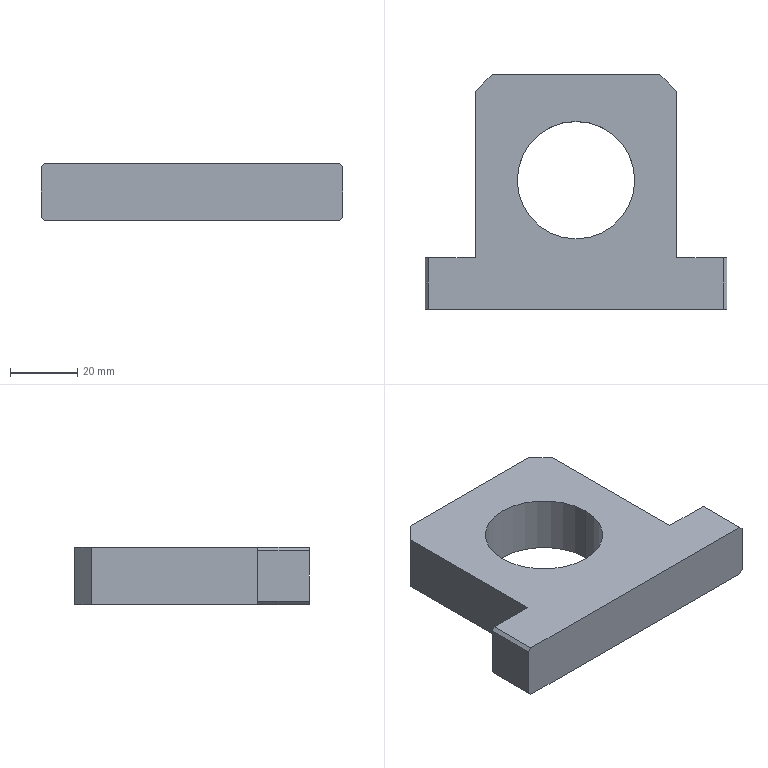Part | STEP file | 001-009-Riveting mechanism cylinder mounting plate | 1 solid | 18 faces | box 90.002 x 70 x 17 mm | volume 62443 mm3 | plane 16 | cylinder 2 | commonest cylinder face diameters 35 x2
STEP:
#1=CARTESIAN_POINT('',(0.,0.,0.));
#2=DIRECTION('',(0.,0.,1.));
#3=DIRECTION('',(1.,0.,0.));
#4=AXIS2_PLACEMENT_3D('',#1,#2,#3);
#5=CARTESIAN_POINT('',(17.5,30.801,0.));
#6=VERTEX_POINT('',#5);
#7=CARTESIAN_POINT('',(17.5,30.801,17.));
#8=VERTEX_POINT('',#7);
#9=CARTESIAN_POINT('',(17.5,30.801,0.));
#10=DIRECTION('',(0.,0.,1.));
#11=VECTOR('',#10,1.);
#12=LINE('',#9,#11);
#13=CARTESIAN_POINT('',(0.,30.801,0.));
#14=DIRECTION('',(0.,0.,1.));
#15=DIRECTION('',(1.,0.,0.));
#16=AXIS2_PLACEMENT_3D('',#13,#14,#15);
#17=CYLINDRICAL_SURFACE('',#16,17.5);
#18=CARTESIAN_POINT('',(6.283,0.));
#19=DIRECTION('',(0.,1.));
#20=VECTOR('',#19,1.);
#21=LINE('',#18,#20);
#22=(GEOMETRIC_REPRESENTATION_CONTEXT(2)PARAMETRIC_REPRESENTATION_CONTEXT()REPRESENTATION_CONTEXT('',''));
#23=DEFINITIONAL_REPRESENTATION('',(#21),#22);
#24=PCURVE('',#17,#23);
#25=CARTESIAN_POINT('',(0.,30.801,0.));
#26=DIRECTION('',(0.,0.,1.));
#27=DIRECTION('',(1.,0.,0.));
#28=AXIS2_PLACEMENT_3D('',#25,#26,#27);
#29=CYLINDRICAL_SURFACE('',#28,17.5);
#30=CARTESIAN_POINT('',(0.,0.));
#31=DIRECTION('',(0.,1.));
#32=VECTOR('',#31,1.);
#33=LINE('',#30,#32);
#34=(GEOMETRIC_REPRESENTATION_CONTEXT(2)PARAMETRIC_REPRESENTATION_CONTEXT()REPRESENTATION_CONTEXT('',''));
#35=DEFINITIONAL_REPRESENTATION('',(#33),#34);
#36=PCURVE('',#29,#35);
#37=SURFACE_CURVE('',#12,(#24,#36),.PCURVE_S1.);
#38=EDGE_CURVE('',#6,#8,#37,.T.);
#39=ORIENTED_EDGE('',*,*,#38,.T.);
#40=CARTESIAN_POINT('',(-17.5,30.801,17.));
#41=VERTEX_POINT('',#40);
#42=CARTESIAN_POINT('',(0.,30.801,17.));
#43=DIRECTION('',(0.,0.,1.));
#44=DIRECTION('',(1.,0.,0.));
#45=AXIS2_PLACEMENT_3D('',#42,#43,#44);
#46=CIRCLE('',#45,17.5);
#47=CARTESIAN_POINT('',(0.,17.));
#48=DIRECTION('',(1.,0.));
#49=VECTOR('',#48,1.);
#50=LINE('',#47,#49);
#51=(GEOMETRIC_REPRESENTATION_CONTEXT(2)PARAMETRIC_REPRESENTATION_CONTEXT()REPRESENTATION_CONTEXT('',''));
#52=DEFINITIONAL_REPRESENTATION('',(#50),#51);
#53=PCURVE('',#17,#52);
#54=CARTESIAN_POINT('',(0.,0.,17.));
#55=DIRECTION('',(0.,0.,1.));
#56=DIRECTION('',(1.,0.,0.));
#57=AXIS2_PLACEMENT_3D('',#54,#55,#56);
#58=PLANE('',#57);
#59=CARTESIAN_POINT('',(0.,30.801));
#60=DIRECTION('',(1.,0.));
#61=AXIS2_PLACEMENT_2D('',#59,#60);
#62=CIRCLE('',#61,17.5);
#63=(GEOMETRIC_REPRESENTATION_CONTEXT(2)PARAMETRIC_REPRESENTATION_CONTEXT()REPRESENTATION_CONTEXT('',''));
#64=DEFINITIONAL_REPRESENTATION('',(#62),#63);
#65=PCURVE('',#58,#64);
#66=SURFACE_CURVE('',#46,(#53,#65),.PCURVE_S1.);
#67=EDGE_CURVE('',#41,#8,#66,.T.);
#68=ORIENTED_EDGE('',*,*,#67,.F.);
#69=CARTESIAN_POINT('',(-17.5,30.801,0.));
#70=VERTEX_POINT('',#69);
#71=CARTESIAN_POINT('',(-17.5,30.801,0.));
#72=DIRECTION('',(0.,0.,1.));
#73=VECTOR('',#72,1.);
#74=LINE('',#71,#73);
#75=CARTESIAN_POINT('',(3.142,0.));
#76=DIRECTION('',(0.,1.));
#77=VECTOR('',#76,1.);
#78=LINE('',#75,#77);
#79=(GEOMETRIC_REPRESENTATION_CONTEXT(2)PARAMETRIC_REPRESENTATION_CONTEXT()REPRESENTATION_CONTEXT('',''));
#80=DEFINITIONAL_REPRESENTATION('',(#78),#79);
#81=PCURVE('',#17,#80);
#82=CARTESIAN_POINT('',(3.142,0.));
#83=DIRECTION('',(0.,1.));
#84=VECTOR('',#83,1.);
#85=LINE('',#82,#84);
#86=(GEOMETRIC_REPRESENTATION_CONTEXT(2)PARAMETRIC_REPRESENTATION_CONTEXT()REPRESENTATION_CONTEXT('',''));
#87=DEFINITIONAL_REPRESENTATION('',(#85),#86);
#88=PCURVE('',#29,#87);
#89=SURFACE_CURVE('',#74,(#81,#88),.PCURVE_S1.);
#90=EDGE_CURVE('',#70,#41,#89,.T.);
#91=ORIENTED_EDGE('',*,*,#90,.F.);
#92=CARTESIAN_POINT('',(0.,30.801,0.));
#93=DIRECTION('',(0.,0.,1.));
#94=DIRECTION('',(1.,0.,0.));
#95=AXIS2_PLACEMENT_3D('',#92,#93,#94);
#96=CIRCLE('',#95,17.5);
#97=CARTESIAN_POINT('',(0.,0.));
#98=DIRECTION('',(1.,0.));
#99=VECTOR('',#98,1.);
#100=LINE('',#97,#99);
#101=(GEOMETRIC_REPRESENTATION_CONTEXT(2)PARAMETRIC_REPRESENTATION_CONTEXT()REPRESENTATION_CONTEXT('',''));
#102=DEFINITIONAL_REPRESENTATION('',(#100),#101);
#103=PCURVE('',#17,#102);
#104=CARTESIAN_POINT('',(0.,0.,0.));
#105=DIRECTION('',(0.,0.,1.));
#106=DIRECTION('',(1.,0.,0.));
#107=AXIS2_PLACEMENT_3D('',#104,#105,#106);
#108=PLANE('',#107);
#109=CARTESIAN_POINT('',(0.,30.801));
#110=DIRECTION('',(1.,0.));
#111=AXIS2_PLACEMENT_2D('',#109,#110);
#112=CIRCLE('',#111,17.5);
#113=(GEOMETRIC_REPRESENTATION_CONTEXT(2)PARAMETRIC_REPRESENTATION_CONTEXT()REPRESENTATION_CONTEXT('',''));
#114=DEFINITIONAL_REPRESENTATION('',(#112),#113);
#115=PCURVE('',#108,#114);
#116=SURFACE_CURVE('',#96,(#103,#115),.PCURVE_S1.);
#117=EDGE_CURVE('',#70,#6,#116,.T.);
#118=ORIENTED_EDGE('',*,*,#117,.T.);
#119=EDGE_LOOP('',(#39,#68,#91,#118));
#120=FACE_BOUND('',#119,.F.);
#121=ADVANCED_FACE('',(#120),#17,.F.);
#122=CARTESIAN_POINT('',(44.001,7.699,17.));
#123=VERTEX_POINT('',#122);
#124=CARTESIAN_POINT('',(30.001,7.699,17.));
#125=VERTEX_POINT('',#124);
#126=CARTESIAN_POINT('',(30.001,7.699,17.));
#127=DIRECTION('',(-1.,0.,0.));
#128=VECTOR('',#127,1.);
#129=LINE('',#126,#128);
#130=CARTESIAN_POINT('',(30.001,7.699,17.));
#131=DIRECTION('',(0.,-1.,0.));
#132=DIRECTION('',(1.,0.,0.));
#133=AXIS2_PLACEMENT_3D('',#130,#131,#132);
#134=PLANE('',#133);
#135=CARTESIAN_POINT('',(0.,0.));
#136=DIRECTION('',(-1.,0.));
#137=VECTOR('',#136,1.);
#138=LINE('',#135,#137);
#139=(GEOMETRIC_REPRESENTATION_CONTEXT(2)PARAMETRIC_REPRESENTATION_CONTEXT()REPRESENTATION_CONTEXT('',''));
#140=DEFINITIONAL_REPRESENTATION('',(#138),#139);
#141=PCURVE('',#134,#140);
#142=CARTESIAN_POINT('',(30.001,7.699));
#143=DIRECTION('',(-1.,0.));
#144=VECTOR('',#143,1.);
#145=LINE('',#142,#144);
#146=(GEOMETRIC_REPRESENTATION_CONTEXT(2)PARAMETRIC_REPRESENTATION_CONTEXT()REPRESENTATION_CONTEXT('',''));
#147=DEFINITIONAL_REPRESENTATION('',(#145),#146);
#148=PCURVE('',#58,#147);
#149=SURFACE_CURVE('',#129,(#141,#148),.PCURVE_S1.);
#150=EDGE_CURVE('',#123,#125,#149,.T.);
#151=ORIENTED_EDGE('',*,*,#150,.F.);
#152=CARTESIAN_POINT('',(45.001,7.699,16.));
#153=VERTEX_POINT('',#152);
#154=CARTESIAN_POINT('',(44.001,7.699,17.));
#155=DIRECTION('',(0.7071,0.,-0.7071));
#156=VECTOR('',#155,1.);
#157=LINE('',#154,#156);
#158=CARTESIAN_POINT('',(14.,0.));
#159=DIRECTION('',(0.7071,-0.7071));
#160=VECTOR('',#159,1.);
#161=LINE('',#158,#160);
#162=(GEOMETRIC_REPRESENTATION_CONTEXT(2)PARAMETRIC_REPRESENTATION_CONTEXT()REPRESENTATION_CONTEXT('',''));
#163=DEFINITIONAL_REPRESENTATION('',(#161),#162);
#164=PCURVE('',#134,#163);
#165=CARTESIAN_POINT('',(44.001,0.,17.));
#166=DIRECTION('',(0.7071,0.,0.7071));
#167=DIRECTION('',(0.,-1.,0.));
#168=AXIS2_PLACEMENT_3D('',#165,#166,#167);
#169=PLANE('',#168);
#170=CARTESIAN_POINT('',(-7.699,0.));
#171=DIRECTION('',(0.,1.));
#172=VECTOR('',#171,1.);
#173=LINE('',#170,#172);
#174=(GEOMETRIC_REPRESENTATION_CONTEXT(2)PARAMETRIC_REPRESENTATION_CONTEXT()REPRESENTATION_CONTEXT('',''));
#175=DEFINITIONAL_REPRESENTATION('',(#173),#174);
#176=PCURVE('',#169,#175);
#177=SURFACE_CURVE('',#157,(#164,#176),.PCURVE_S1.);
#178=EDGE_CURVE('',#123,#153,#177,.T.);
#179=ORIENTED_EDGE('',*,*,#178,.T.);
#180=CARTESIAN_POINT('',(45.001,7.699,1.));
#181=VERTEX_POINT('',#180);
#182=CARTESIAN_POINT('',(45.001,7.699,17.));
#183=DIRECTION('',(0.,0.,-1.));
#184=VECTOR('',#183,1.);
#185=LINE('',#182,#184);
#186=CARTESIAN_POINT('',(15.,0.));
#187=DIRECTION('',(0.,-1.));
#188=VECTOR('',#187,1.);
#189=LINE('',#186,#188);
#190=(GEOMETRIC_REPRESENTATION_CONTEXT(2)PARAMETRIC_REPRESENTATION_CONTEXT()REPRESENTATION_CONTEXT('',''));
#191=DEFINITIONAL_REPRESENTATION('',(#189),#190);
#192=PCURVE('',#134,#191);
#193=CARTESIAN_POINT('',(45.001,-7.699,17.));
#194=DIRECTION('',(-1.,0.,0.));
#195=DIRECTION('',(0.,0.,1.));
#196=AXIS2_PLACEMENT_3D('',#193,#194,#195);
#197=PLANE('',#196);
#198=CARTESIAN_POINT('',(0.,15.397));
#199=DIRECTION('',(-1.,0.));
#200=VECTOR('',#199,1.);
#201=LINE('',#198,#200);
#202=(GEOMETRIC_REPRESENTATION_CONTEXT(2)PARAMETRIC_REPRESENTATION_CONTEXT()REPRESENTATION_CONTEXT('',''));
#203=DEFINITIONAL_REPRESENTATION('',(#201),#202);
#204=PCURVE('',#197,#203);
#205=SURFACE_CURVE('',#185,(#192,#204),.PCURVE_S1.);
#206=EDGE_CURVE('',#153,#181,#205,.T.);
#207=ORIENTED_EDGE('',*,*,#206,.T.);
#208=CARTESIAN_POINT('',(44.001,7.699,0.));
#209=VERTEX_POINT('',#208);
#210=CARTESIAN_POINT('',(45.001,7.699,1.));
#211=DIRECTION('',(-0.7071,0.,-0.7071));
#212=VECTOR('',#211,1.);
#213=LINE('',#210,#212);
#214=CARTESIAN_POINT('',(15.,-16.));
#215=DIRECTION('',(-0.7071,-0.7071));
#216=VECTOR('',#215,1.);
#217=LINE('',#214,#216);
#218=(GEOMETRIC_REPRESENTATION_CONTEXT(2)PARAMETRIC_REPRESENTATION_CONTEXT()REPRESENTATION_CONTEXT('',''));
#219=DEFINITIONAL_REPRESENTATION('',(#217),#218);
#220=PCURVE('',#134,#219);
#221=CARTESIAN_POINT('',(45.001,-7.699,1.));
#222=DIRECTION('',(-0.7071,0.,0.7071));
#223=DIRECTION('',(0.,1.,0.));
#224=AXIS2_PLACEMENT_3D('',#221,#222,#223);
#225=PLANE('',#224);
#226=CARTESIAN_POINT('',(15.397,0.));
#227=DIRECTION('',(0.,1.));
#228=VECTOR('',#227,1.);
#229=LINE('',#226,#228);
#230=(GEOMETRIC_REPRESENTATION_CONTEXT(2)PARAMETRIC_REPRESENTATION_CONTEXT()REPRESENTATION_CONTEXT('',''));
#231=DEFINITIONAL_REPRESENTATION('',(#229),#230);
#232=PCURVE('',#225,#231);
#233=SURFACE_CURVE('',#213,(#220,#232),.PCURVE_S1.);
#234=EDGE_CURVE('',#181,#209,#233,.T.);
#235=ORIENTED_EDGE('',*,*,#234,.T.);
#236=CARTESIAN_POINT('',(30.001,7.699,0.));
#237=VERTEX_POINT('',#236);
#238=CARTESIAN_POINT('',(30.001,7.699,0.));
#239=DIRECTION('',(-1.,0.,0.));
#240=VECTOR('',#239,1.);
#241=LINE('',#238,#240);
#242=CARTESIAN_POINT('',(0.,-17.));
#243=DIRECTION('',(-1.,0.));
#244=VECTOR('',#243,1.);
#245=LINE('',#242,#244);
#246=(GEOMETRIC_REPRESENTATION_CONTEXT(2)PARAMETRIC_REPRESENTATION_CONTEXT()REPRESENTATION_CONTEXT('',''));
#247=DEFINITIONAL_REPRESENTATION('',(#245),#246);
#248=PCURVE('',#134,#247);
#249=CARTESIAN_POINT('',(30.001,7.699));
#250=DIRECTION('',(-1.,0.));
#251=VECTOR('',#250,1.);
#252=LINE('',#249,#251);
#253=(GEOMETRIC_REPRESENTATION_CONTEXT(2)PARAMETRIC_REPRESENTATION_CONTEXT()REPRESENTATION_CONTEXT('',''));
#254=DEFINITIONAL_REPRESENTATION('',(#252),#253);
#255=PCURVE('',#108,#254);
#256=SURFACE_CURVE('',#241,(#248,#255),.PCURVE_S1.);
#257=EDGE_CURVE('',#209,#237,#256,.T.);
#258=ORIENTED_EDGE('',*,*,#257,.T.);
#259=CARTESIAN_POINT('',(30.001,7.699,17.));
#260=DIRECTION('',(0.,0.,-1.));
#261=VECTOR('',#260,1.);
#262=LINE('',#259,#261);
#263=CARTESIAN_POINT('',(0.,0.));
#264=DIRECTION('',(0.,-1.));
#265=VECTOR('',#264,1.);
#266=LINE('',#263,#265);
#267=(GEOMETRIC_REPRESENTATION_CONTEXT(2)PARAMETRIC_REPRESENTATION_CONTEXT()REPRESENTATION_CONTEXT('',''));
#268=DEFINITIONAL_REPRESENTATION('',(#266),#267);
#269=PCURVE('',#134,#268);
#270=CARTESIAN_POINT('',(30.001,7.699,17.));
#271=DIRECTION('',(-1.,0.,0.));
#272=DIRECTION('',(0.,-1.,0.));
#273=AXIS2_PLACEMENT_3D('',#270,#271,#272);
#274=PLANE('',#273);
#275=CARTESIAN_POINT('',(0.,0.));
#276=DIRECTION('',(0.,-1.));
#277=VECTOR('',#276,1.);
#278=LINE('',#275,#277);
#279=(GEOMETRIC_REPRESENTATION_CONTEXT(2)PARAMETRIC_REPRESENTATION_CONTEXT()REPRESENTATION_CONTEXT('',''));
#280=DEFINITIONAL_REPRESENTATION('',(#278),#279);
#281=PCURVE('',#274,#280);
#282=SURFACE_CURVE('',#262,(#269,#281),.PCURVE_S1.);
#283=EDGE_CURVE('',#125,#237,#282,.T.);
#284=ORIENTED_EDGE('',*,*,#283,.F.);
#285=EDGE_LOOP('',(#151,#179,#207,#235,#258,#284));
#286=FACE_BOUND('',#285,.T.);
#287=ADVANCED_FACE('',(#286),#134,.F.);
#288=CARTESIAN_POINT('',(30.001,57.301,0.));
#289=VERTEX_POINT('',#288);
#290=CARTESIAN_POINT('',(30.001,7.699,0.));
#291=DIRECTION('',(0.,1.,0.));
#292=VECTOR('',#291,1.);
#293=LINE('',#290,#292);
#294=CARTESIAN_POINT('',(0.,-17.));
#295=DIRECTION('',(-1.,0.));
#296=VECTOR('',#295,1.);
#297=LINE('',#294,#296);
#298=(GEOMETRIC_REPRESENTATION_CONTEXT(2)PARAMETRIC_REPRESENTATION_CONTEXT()REPRESENTATION_CONTEXT('',''));
#299=DEFINITIONAL_REPRESENTATION('',(#297),#298);
#300=PCURVE('',#274,#299);
#301=CARTESIAN_POINT('',(30.001,7.699));
#302=DIRECTION('',(0.,1.));
#303=VECTOR('',#302,1.);
#304=LINE('',#301,#303);
#305=(GEOMETRIC_REPRESENTATION_CONTEXT(2)PARAMETRIC_REPRESENTATION_CONTEXT()REPRESENTATION_CONTEXT('',''));
#306=DEFINITIONAL_REPRESENTATION('',(#304),#305);
#307=PCURVE('',#108,#306);
#308=SURFACE_CURVE('',#293,(#300,#307),.PCURVE_S1.);
#309=EDGE_CURVE('',#237,#289,#308,.T.);
#310=ORIENTED_EDGE('',*,*,#309,.T.);
#311=CARTESIAN_POINT('',(30.001,57.301,17.));
#312=VERTEX_POINT('',#311);
#313=CARTESIAN_POINT('',(30.001,57.301,17.));
#314=DIRECTION('',(0.,0.,1.));
#315=VECTOR('',#314,1.);
#316=LINE('',#313,#315);
#317=CARTESIAN_POINT('',(-49.603,0.));
#318=DIRECTION('',(0.,1.));
#319=VECTOR('',#318,1.);
#320=LINE('',#317,#319);
#321=(GEOMETRIC_REPRESENTATION_CONTEXT(2)PARAMETRIC_REPRESENTATION_CONTEXT()REPRESENTATION_CONTEXT('',''));
#322=DEFINITIONAL_REPRESENTATION('',(#320),#321);
#323=PCURVE('',#274,#322);
#324=CARTESIAN_POINT('',(25.001,62.301,17.));
#325=DIRECTION('',(-0.7071,-0.7071,0.));
#326=DIRECTION('',(0.,0.,-1.));
#327=AXIS2_PLACEMENT_3D('',#324,#325,#326);
#328=PLANE('',#327);
#329=CARTESIAN_POINT('',(0.,7.071));
#330=DIRECTION('',(-1.,0.));
#331=VECTOR('',#330,1.);
#332=LINE('',#329,#331);
#333=(GEOMETRIC_REPRESENTATION_CONTEXT(2)PARAMETRIC_REPRESENTATION_CONTEXT()REPRESENTATION_CONTEXT('',''));
#334=DEFINITIONAL_REPRESENTATION('',(#332),#333);
#335=PCURVE('',#328,#334);
#336=SURFACE_CURVE('',#316,(#323,#335),.PCURVE_S1.);
#337=EDGE_CURVE('',#289,#312,#336,.T.);
#338=ORIENTED_EDGE('',*,*,#337,.T.);
#339=CARTESIAN_POINT('',(30.001,7.699,17.));
#340=DIRECTION('',(0.,1.,0.));
#341=VECTOR('',#340,1.);
#342=LINE('',#339,#341);
#343=CARTESIAN_POINT('',(0.,0.));
#344=DIRECTION('',(-1.,0.));
#345=VECTOR('',#344,1.);
#346=LINE('',#343,#345);
#347=(GEOMETRIC_REPRESENTATION_CONTEXT(2)PARAMETRIC_REPRESENTATION_CONTEXT()REPRESENTATION_CONTEXT('',''));
#348=DEFINITIONAL_REPRESENTATION('',(#346),#347);
#349=PCURVE('',#274,#348);
#350=CARTESIAN_POINT('',(30.001,7.699));
#351=DIRECTION('',(0.,1.));
#352=VECTOR('',#351,1.);
#353=LINE('',#350,#352);
#354=(GEOMETRIC_REPRESENTATION_CONTEXT(2)PARAMETRIC_REPRESENTATION_CONTEXT()REPRESENTATION_CONTEXT('',''));
#355=DEFINITIONAL_REPRESENTATION('',(#353),#354);
#356=PCURVE('',#58,#355);
#357=SURFACE_CURVE('',#342,(#349,#356),.PCURVE_S1.);
#358=EDGE_CURVE('',#125,#312,#357,.T.);
#359=ORIENTED_EDGE('',*,*,#358,.F.);
#360=ORIENTED_EDGE('',*,*,#283,.T.);
#361=EDGE_LOOP('',(#310,#338,#359,#360));
#362=FACE_BOUND('',#361,.T.);
#363=ADVANCED_FACE('',(#362),#274,.F.);
#364=CARTESIAN_POINT('',(25.001,62.301,0.));
#365=VERTEX_POINT('',#364);
#366=CARTESIAN_POINT('',(-25.001,62.301,0.));
#367=VERTEX_POINT('',#366);
#368=CARTESIAN_POINT('',(-30.001,62.301,0.));
#369=DIRECTION('',(-1.,0.,0.));
#370=VECTOR('',#369,1.);
#371=LINE('',#368,#370);
#372=CARTESIAN_POINT('',(-30.001,62.301,17.));
#373=DIRECTION('',(0.,-1.,0.));
#374=DIRECTION('',(0.,0.,-1.));
#375=AXIS2_PLACEMENT_3D('',#372,#373,#374);
#376=PLANE('',#375);
#377=CARTESIAN_POINT('',(17.,0.));
#378=DIRECTION('',(0.,-1.));
#379=VECTOR('',#378,1.);
#380=LINE('',#377,#379);
#381=(GEOMETRIC_REPRESENTATION_CONTEXT(2)PARAMETRIC_REPRESENTATION_CONTEXT()REPRESENTATION_CONTEXT('',''));
#382=DEFINITIONAL_REPRESENTATION('',(#380),#381);
#383=PCURVE('',#376,#382);
#384=CARTESIAN_POINT('',(-30.001,62.301));
#385=DIRECTION('',(-1.,0.));
#386=VECTOR('',#385,1.);
#387=LINE('',#384,#386);
#388=(GEOMETRIC_REPRESENTATION_CONTEXT(2)PARAMETRIC_REPRESENTATION_CONTEXT()REPRESENTATION_CONTEXT('',''));
#389=DEFINITIONAL_REPRESENTATION('',(#387),#388);
#390=PCURVE('',#108,#389);
#391=SURFACE_CURVE('',#371,(#383,#390),.PCURVE_S1.);
#392=EDGE_CURVE('',#365,#367,#391,.T.);
#393=ORIENTED_EDGE('',*,*,#392,.T.);
#394=CARTESIAN_POINT('',(-25.001,62.301,17.));
#395=VERTEX_POINT('',#394);
#396=CARTESIAN_POINT('',(-25.001,62.301,17.));
#397=DIRECTION('',(0.,0.,1.));
#398=VECTOR('',#397,1.);
#399=LINE('',#396,#398);
#400=CARTESIAN_POINT('',(0.,5.));
#401=DIRECTION('',(-1.,0.));
#402=VECTOR('',#401,1.);
#403=LINE('',#400,#402);
#404=(GEOMETRIC_REPRESENTATION_CONTEXT(2)PARAMETRIC_REPRESENTATION_CONTEXT()REPRESENTATION_CONTEXT('',''));
#405=DEFINITIONAL_REPRESENTATION('',(#403),#404);
#406=PCURVE('',#376,#405);
#407=CARTESIAN_POINT('',(-30.001,57.301,17.));
#408=DIRECTION('',(0.7071,-0.7071,0.));
#409=DIRECTION('',(0.,0.,-1.));
#410=AXIS2_PLACEMENT_3D('',#407,#408,#409);
#411=PLANE('',#410);
#412=CARTESIAN_POINT('',(0.,7.071));
#413=DIRECTION('',(-1.,0.));
#414=VECTOR('',#413,1.);
#415=LINE('',#412,#414);
#416=(GEOMETRIC_REPRESENTATION_CONTEXT(2)PARAMETRIC_REPRESENTATION_CONTEXT()REPRESENTATION_CONTEXT('',''));
#417=DEFINITIONAL_REPRESENTATION('',(#415),#416);
#418=PCURVE('',#411,#417);
#419=SURFACE_CURVE('',#399,(#406,#418),.PCURVE_S1.);
#420=EDGE_CURVE('',#367,#395,#419,.T.);
#421=ORIENTED_EDGE('',*,*,#420,.T.);
#422=CARTESIAN_POINT('',(25.001,62.301,17.));
#423=VERTEX_POINT('',#422);
#424=CARTESIAN_POINT('',(-30.001,62.301,17.));
#425=DIRECTION('',(-1.,0.,0.));
#426=VECTOR('',#425,1.);
#427=LINE('',#424,#426);
#428=CARTESIAN_POINT('',(0.,0.));
#429=DIRECTION('',(0.,-1.));
#430=VECTOR('',#429,1.);
#431=LINE('',#428,#430);
#432=(GEOMETRIC_REPRESENTATION_CONTEXT(2)PARAMETRIC_REPRESENTATION_CONTEXT()REPRESENTATION_CONTEXT('',''));
#433=DEFINITIONAL_REPRESENTATION('',(#431),#432);
#434=PCURVE('',#376,#433);
#435=CARTESIAN_POINT('',(-30.001,62.301));
#436=DIRECTION('',(-1.,0.));
#437=VECTOR('',#436,1.);
#438=LINE('',#435,#437);
#439=(GEOMETRIC_REPRESENTATION_CONTEXT(2)PARAMETRIC_REPRESENTATION_CONTEXT()REPRESENTATION_CONTEXT('',''));
#440=DEFINITIONAL_REPRESENTATION('',(#438),#439);
#441=PCURVE('',#58,#440);
#442=SURFACE_CURVE('',#427,(#434,#441),.PCURVE_S1.);
#443=EDGE_CURVE('',#423,#395,#442,.T.);
#444=ORIENTED_EDGE('',*,*,#443,.F.);
#445=CARTESIAN_POINT('',(25.001,62.301,17.));
#446=DIRECTION('',(0.,0.,-1.));
#447=VECTOR('',#446,1.);
#448=LINE('',#445,#447);
#449=CARTESIAN_POINT('',(0.,55.002));
#450=DIRECTION('',(1.,0.));
#451=VECTOR('',#450,1.);
#452=LINE('',#449,#451);
#453=(GEOMETRIC_REPRESENTATION_CONTEXT(2)PARAMETRIC_REPRESENTATION_CONTEXT()REPRESENTATION_CONTEXT('',''));
#454=DEFINITIONAL_REPRESENTATION('',(#452),#453);
#455=PCURVE('',#376,#454);
#456=CARTESIAN_POINT('',(0.,0.));
#457=DIRECTION('',(1.,0.));
#458=VECTOR('',#457,1.);
#459=LINE('',#456,#458);
#460=(GEOMETRIC_REPRESENTATION_CONTEXT(2)PARAMETRIC_REPRESENTATION_CONTEXT()REPRESENTATION_CONTEXT('',''));
#461=DEFINITIONAL_REPRESENTATION('',(#459),#460);
#462=PCURVE('',#328,#461);
#463=SURFACE_CURVE('',#448,(#455,#462),.PCURVE_S1.);
#464=EDGE_CURVE('',#423,#365,#463,.T.);
#465=ORIENTED_EDGE('',*,*,#464,.T.);
#466=EDGE_LOOP('',(#393,#421,#444,#465));
#467=FACE_BOUND('',#466,.T.);
#468=ADVANCED_FACE('',(#467),#376,.F.);
#469=CARTESIAN_POINT('',(-30.001,57.301,17.));
#470=VERTEX_POINT('',#469);
#471=CARTESIAN_POINT('',(-30.001,7.699,17.));
#472=VERTEX_POINT('',#471);
#473=CARTESIAN_POINT('',(-30.001,7.699,17.));
#474=DIRECTION('',(0.,-1.,0.));
#475=VECTOR('',#474,1.);
#476=LINE('',#473,#475);
#477=CARTESIAN_POINT('',(-30.001,7.699,17.));
#478=DIRECTION('',(1.,0.,0.));
#479=DIRECTION('',(0.,1.,0.));
#480=AXIS2_PLACEMENT_3D('',#477,#478,#479);
#481=PLANE('',#480);
#482=CARTESIAN_POINT('',(0.,0.));
#483=DIRECTION('',(-1.,0.));
#484=VECTOR('',#483,1.);
#485=LINE('',#482,#484);
#486=(GEOMETRIC_REPRESENTATION_CONTEXT(2)PARAMETRIC_REPRESENTATION_CONTEXT()REPRESENTATION_CONTEXT('',''));
#487=DEFINITIONAL_REPRESENTATION('',(#485),#486);
#488=PCURVE('',#481,#487);
#489=CARTESIAN_POINT('',(-30.001,7.699));
#490=DIRECTION('',(0.,-1.));
#491=VECTOR('',#490,1.);
#492=LINE('',#489,#491);
#493=(GEOMETRIC_REPRESENTATION_CONTEXT(2)PARAMETRIC_REPRESENTATION_CONTEXT()REPRESENTATION_CONTEXT('',''));
#494=DEFINITIONAL_REPRESENTATION('',(#492),#493);
#495=PCURVE('',#58,#494);
#496=SURFACE_CURVE('',#476,(#488,#495),.PCURVE_S1.);
#497=EDGE_CURVE('',#470,#472,#496,.T.);
#498=ORIENTED_EDGE('',*,*,#497,.F.);
#499=CARTESIAN_POINT('',(-30.001,57.301,0.));
#500=VERTEX_POINT('',#499);
#501=CARTESIAN_POINT('',(-30.001,57.301,17.));
#502=DIRECTION('',(0.,0.,-1.));
#503=VECTOR('',#502,1.);
#504=LINE('',#501,#503);
#505=CARTESIAN_POINT('',(49.603,0.));
#506=DIRECTION('',(0.,-1.));
#507=VECTOR('',#506,1.);
#508=LINE('',#505,#507);
#509=(GEOMETRIC_REPRESENTATION_CONTEXT(2)PARAMETRIC_REPRESENTATION_CONTEXT()REPRESENTATION_CONTEXT('',''));
#510=DEFINITIONAL_REPRESENTATION('',(#508),#509);
#511=PCURVE('',#481,#510);
#512=CARTESIAN_POINT('',(0.,0.));
#513=DIRECTION('',(1.,0.));
#514=VECTOR('',#513,1.);
#515=LINE('',#512,#514);
#516=(GEOMETRIC_REPRESENTATION_CONTEXT(2)PARAMETRIC_REPRESENTATION_CONTEXT()REPRESENTATION_CONTEXT('',''));
#517=DEFINITIONAL_REPRESENTATION('',(#515),#516);
#518=PCURVE('',#411,#517);
#519=SURFACE_CURVE('',#504,(#511,#518),.PCURVE_S1.);
#520=EDGE_CURVE('',#470,#500,#519,.T.);
#521=ORIENTED_EDGE('',*,*,#520,.T.);
#522=CARTESIAN_POINT('',(-30.001,7.699,0.));
#523=VERTEX_POINT('',#522);
#524=CARTESIAN_POINT('',(-30.001,7.699,0.));
#525=DIRECTION('',(0.,-1.,0.));
#526=VECTOR('',#525,1.);
#527=LINE('',#524,#526);
#528=CARTESIAN_POINT('',(0.,-17.));
#529=DIRECTION('',(-1.,0.));
#530=VECTOR('',#529,1.);
#531=LINE('',#528,#530);
#532=(GEOMETRIC_REPRESENTATION_CONTEXT(2)PARAMETRIC_REPRESENTATION_CONTEXT()REPRESENTATION_CONTEXT('',''));
#533=DEFINITIONAL_REPRESENTATION('',(#531),#532);
#534=PCURVE('',#481,#533);
#535=CARTESIAN_POINT('',(-30.001,7.699));
#536=DIRECTION('',(0.,-1.));
#537=VECTOR('',#536,1.);
#538=LINE('',#535,#537);
#539=(GEOMETRIC_REPRESENTATION_CONTEXT(2)PARAMETRIC_REPRESENTATION_CONTEXT()REPRESENTATION_CONTEXT('',''));
#540=DEFINITIONAL_REPRESENTATION('',(#538),#539);
#541=PCURVE('',#108,#540);
#542=SURFACE_CURVE('',#527,(#534,#541),.PCURVE_S1.);
#543=EDGE_CURVE('',#500,#523,#542,.T.);
#544=ORIENTED_EDGE('',*,*,#543,.T.);
#545=CARTESIAN_POINT('',(-30.001,7.699,17.));
#546=DIRECTION('',(0.,0.,-1.));
#547=VECTOR('',#546,1.);
#548=LINE('',#545,#547);
#549=CARTESIAN_POINT('',(0.,0.));
#550=DIRECTION('',(0.,-1.));
#551=VECTOR('',#550,1.);
#552=LINE('',#549,#551);
#553=(GEOMETRIC_REPRESENTATION_CONTEXT(2)PARAMETRIC_REPRESENTATION_CONTEXT()REPRESENTATION_CONTEXT('',''));
#554=DEFINITIONAL_REPRESENTATION('',(#552),#553);
#555=PCURVE('',#481,#554);
#556=CARTESIAN_POINT('',(-45.001,7.699,17.));
#557=DIRECTION('',(0.,-1.,0.));
#558=DIRECTION('',(1.,0.,0.));
#559=AXIS2_PLACEMENT_3D('',#556,#557,#558);
#560=PLANE('',#559);
#561=CARTESIAN_POINT('',(15.,0.));
#562=DIRECTION('',(0.,-1.));
#563=VECTOR('',#562,1.);
#564=LINE('',#561,#563);
#565=(GEOMETRIC_REPRESENTATION_CONTEXT(2)PARAMETRIC_REPRESENTATION_CONTEXT()REPRESENTATION_CONTEXT('',''));
#566=DEFINITIONAL_REPRESENTATION('',(#564),#565);
#567=PCURVE('',#560,#566);
#568=SURFACE_CURVE('',#548,(#555,#567),.PCURVE_S1.);
#569=EDGE_CURVE('',#472,#523,#568,.T.);
#570=ORIENTED_EDGE('',*,*,#569,.F.);
#571=EDGE_LOOP('',(#498,#521,#544,#570));
#572=FACE_BOUND('',#571,.T.);
#573=ADVANCED_FACE('',(#572),#481,.F.);
#574=CARTESIAN_POINT('',(-44.001,7.699,0.));
#575=VERTEX_POINT('',#574);
#576=CARTESIAN_POINT('',(-45.001,7.699,0.));
#577=DIRECTION('',(-1.,0.,0.));
#578=VECTOR('',#577,1.);
#579=LINE('',#576,#578);
#580=CARTESIAN_POINT('',(0.,-17.));
#581=DIRECTION('',(-1.,0.));
#582=VECTOR('',#581,1.);
#583=LINE('',#580,#582);
#584=(GEOMETRIC_REPRESENTATION_CONTEXT(2)PARAMETRIC_REPRESENTATION_CONTEXT()REPRESENTATION_CONTEXT('',''));
#585=DEFINITIONAL_REPRESENTATION('',(#583),#584);
#586=PCURVE('',#560,#585);
#587=CARTESIAN_POINT('',(-45.001,7.699));
#588=DIRECTION('',(-1.,0.));
#589=VECTOR('',#588,1.);
#590=LINE('',#587,#589);
#591=(GEOMETRIC_REPRESENTATION_CONTEXT(2)PARAMETRIC_REPRESENTATION_CONTEXT()REPRESENTATION_CONTEXT('',''));
#592=DEFINITIONAL_REPRESENTATION('',(#590),#591);
#593=PCURVE('',#108,#592);
#594=SURFACE_CURVE('',#579,(#586,#593),.PCURVE_S1.);
#595=EDGE_CURVE('',#523,#575,#594,.T.);
#596=ORIENTED_EDGE('',*,*,#595,.T.);
#597=CARTESIAN_POINT('',(-45.001,7.699,1.));
#598=VERTEX_POINT('',#597);
#599=CARTESIAN_POINT('',(-45.001,7.699,1.));
#600=DIRECTION('',(-0.7071,0.,0.7071));
#601=VECTOR('',#600,1.);
#602=LINE('',#599,#601);
#603=CARTESIAN_POINT('',(0.,-16.));
#604=DIRECTION('',(-0.7071,0.7071));
#605=VECTOR('',#604,1.);
#606=LINE('',#603,#605);
#607=(GEOMETRIC_REPRESENTATION_CONTEXT(2)PARAMETRIC_REPRESENTATION_CONTEXT()REPRESENTATION_CONTEXT('',''));
#608=DEFINITIONAL_REPRESENTATION('',(#606),#607);
#609=PCURVE('',#560,#608);
#610=CARTESIAN_POINT('',(-45.001,-7.699,1.));
#611=DIRECTION('',(0.7071,0.,0.7071));
#612=DIRECTION('',(0.,-1.,0.));
#613=AXIS2_PLACEMENT_3D('',#610,#611,#612);
#614=PLANE('',#613);
#615=CARTESIAN_POINT('',(-15.397,0.));
#616=DIRECTION('',(0.,-1.));
#617=VECTOR('',#616,1.);
#618=LINE('',#615,#617);
#619=(GEOMETRIC_REPRESENTATION_CONTEXT(2)PARAMETRIC_REPRESENTATION_CONTEXT()REPRESENTATION_CONTEXT('',''));
#620=DEFINITIONAL_REPRESENTATION('',(#618),#619);
#621=PCURVE('',#614,#620);
#622=SURFACE_CURVE('',#602,(#609,#621),.PCURVE_S1.);
#623=EDGE_CURVE('',#575,#598,#622,.T.);
#624=ORIENTED_EDGE('',*,*,#623,.T.);
#625=CARTESIAN_POINT('',(-45.001,7.699,16.));
#626=VERTEX_POINT('',#625);
#627=CARTESIAN_POINT('',(-45.001,7.699,17.));
#628=DIRECTION('',(0.,0.,-1.));
#629=VECTOR('',#628,1.);
#630=LINE('',#627,#629);
#631=CARTESIAN_POINT('',(0.,0.));
#632=DIRECTION('',(0.,-1.));
#633=VECTOR('',#632,1.);
#634=LINE('',#631,#633);
#635=(GEOMETRIC_REPRESENTATION_CONTEXT(2)PARAMETRIC_REPRESENTATION_CONTEXT()REPRESENTATION_CONTEXT('',''));
#636=DEFINITIONAL_REPRESENTATION('',(#634),#635);
#637=PCURVE('',#560,#636);
#638=CARTESIAN_POINT('',(-45.001,-7.699,17.));
#639=DIRECTION('',(1.,0.,0.));
#640=DIRECTION('',(0.,0.,-1.));
#641=AXIS2_PLACEMENT_3D('',#638,#639,#640);
#642=PLANE('',#641);
#643=CARTESIAN_POINT('',(0.,15.397));
#644=DIRECTION('',(1.,0.));
#645=VECTOR('',#644,1.);
#646=LINE('',#643,#645);
#647=(GEOMETRIC_REPRESENTATION_CONTEXT(2)PARAMETRIC_REPRESENTATION_CONTEXT()REPRESENTATION_CONTEXT('',''));
#648=DEFINITIONAL_REPRESENTATION('',(#646),#647);
#649=PCURVE('',#642,#648);
#650=SURFACE_CURVE('',#630,(#637,#649),.PCURVE_S1.);
#651=EDGE_CURVE('',#626,#598,#650,.T.);
#652=ORIENTED_EDGE('',*,*,#651,.F.);
#653=CARTESIAN_POINT('',(-44.001,7.699,17.));
#654=VERTEX_POINT('',#653);
#655=CARTESIAN_POINT('',(-44.001,7.699,17.));
#656=DIRECTION('',(0.7071,0.,0.7071));
#657=VECTOR('',#656,1.);
#658=LINE('',#655,#657);
#659=CARTESIAN_POINT('',(1.,0.));
#660=DIRECTION('',(0.7071,0.7071));
#661=VECTOR('',#660,1.);
#662=LINE('',#659,#661);
#663=(GEOMETRIC_REPRESENTATION_CONTEXT(2)PARAMETRIC_REPRESENTATION_CONTEXT()REPRESENTATION_CONTEXT('',''));
#664=DEFINITIONAL_REPRESENTATION('',(#662),#663);
#665=PCURVE('',#560,#664);
#666=CARTESIAN_POINT('',(-44.001,0.,17.));
#667=DIRECTION('',(-0.7071,0.,0.7071));
#668=DIRECTION('',(0.,1.,0.));
#669=AXIS2_PLACEMENT_3D('',#666,#667,#668);
#670=PLANE('',#669);
#671=CARTESIAN_POINT('',(7.699,0.));
#672=DIRECTION('',(0.,-1.));
#673=VECTOR('',#672,1.);
#674=LINE('',#671,#673);
#675=(GEOMETRIC_REPRESENTATION_CONTEXT(2)PARAMETRIC_REPRESENTATION_CONTEXT()REPRESENTATION_CONTEXT('',''));
#676=DEFINITIONAL_REPRESENTATION('',(#674),#675);
#677=PCURVE('',#670,#676);
#678=SURFACE_CURVE('',#658,(#665,#677),.PCURVE_S1.);
#679=EDGE_CURVE('',#626,#654,#678,.T.);
#680=ORIENTED_EDGE('',*,*,#679,.T.);
#681=CARTESIAN_POINT('',(-45.001,7.699,17.));
#682=DIRECTION('',(-1.,0.,0.));
#683=VECTOR('',#682,1.);
#684=LINE('',#681,#683);
#685=CARTESIAN_POINT('',(0.,0.));
#686=DIRECTION('',(-1.,0.));
#687=VECTOR('',#686,1.);
#688=LINE('',#685,#687);
#689=(GEOMETRIC_REPRESENTATION_CONTEXT(2)PARAMETRIC_REPRESENTATION_CONTEXT()REPRESENTATION_CONTEXT('',''));
#690=DEFINITIONAL_REPRESENTATION('',(#688),#689);
#691=PCURVE('',#560,#690);
#692=CARTESIAN_POINT('',(-45.001,7.699));
#693=DIRECTION('',(-1.,0.));
#694=VECTOR('',#693,1.);
#695=LINE('',#692,#694);
#696=(GEOMETRIC_REPRESENTATION_CONTEXT(2)PARAMETRIC_REPRESENTATION_CONTEXT()REPRESENTATION_CONTEXT('',''));
#697=DEFINITIONAL_REPRESENTATION('',(#695),#696);
#698=PCURVE('',#58,#697);
#699=SURFACE_CURVE('',#684,(#691,#698),.PCURVE_S1.);
#700=EDGE_CURVE('',#472,#654,#699,.T.);
#701=ORIENTED_EDGE('',*,*,#700,.F.);
#702=ORIENTED_EDGE('',*,*,#569,.T.);
#703=EDGE_LOOP('',(#596,#624,#652,#680,#701,#702));
#704=FACE_BOUND('',#703,.T.);
#705=ADVANCED_FACE('',(#704),#560,.F.);
#706=ORIENTED_EDGE('',*,*,#651,.T.);
#707=CARTESIAN_POINT('',(-45.001,-7.699,1.));
#708=VERTEX_POINT('',#707);
#709=CARTESIAN_POINT('',(-45.001,-7.699,1.));
#710=DIRECTION('',(0.,-1.,0.));
#711=VECTOR('',#710,1.);
#712=LINE('',#709,#711);
#713=CARTESIAN_POINT('',(16.,0.));
#714=DIRECTION('',(0.,-1.));
#715=VECTOR('',#714,1.);
#716=LINE('',#713,#715);
#717=(GEOMETRIC_REPRESENTATION_CONTEXT(2)PARAMETRIC_REPRESENTATION_CONTEXT()REPRESENTATION_CONTEXT('',''));
#718=DEFINITIONAL_REPRESENTATION('',(#716),#717);
#719=PCURVE('',#642,#718);
#720=CARTESIAN_POINT('',(0.,0.));
#721=DIRECTION('',(1.,0.));
#722=VECTOR('',#721,1.);
#723=LINE('',#720,#722);
#724=(GEOMETRIC_REPRESENTATION_CONTEXT(2)PARAMETRIC_REPRESENTATION_CONTEXT()REPRESENTATION_CONTEXT('',''));
#725=DEFINITIONAL_REPRESENTATION('',(#723),#724);
#726=PCURVE('',#614,#725);
#727=SURFACE_CURVE('',#712,(#719,#726),.PCURVE_S1.);
#728=EDGE_CURVE('',#598,#708,#727,.T.);
#729=ORIENTED_EDGE('',*,*,#728,.T.);
#730=CARTESIAN_POINT('',(-45.001,-7.699,16.));
#731=VERTEX_POINT('',#730);
#732=CARTESIAN_POINT('',(-45.001,-7.699,17.));
#733=DIRECTION('',(0.,0.,-1.));
#734=VECTOR('',#733,1.);
#735=LINE('',#732,#734);
#736=CARTESIAN_POINT('',(0.,0.));
#737=DIRECTION('',(1.,0.));
#738=VECTOR('',#737,1.);
#739=LINE('',#736,#738);
#740=(GEOMETRIC_REPRESENTATION_CONTEXT(2)PARAMETRIC_REPRESENTATION_CONTEXT()REPRESENTATION_CONTEXT('',''));
#741=DEFINITIONAL_REPRESENTATION('',(#739),#740);
#742=PCURVE('',#642,#741);
#743=CARTESIAN_POINT('',(-45.001,-7.699,17.));
#744=DIRECTION('',(0.,1.,0.));
#745=DIRECTION('',(0.,0.,1.));
#746=AXIS2_PLACEMENT_3D('',#743,#744,#745);
#747=PLANE('',#746);
#748=CARTESIAN_POINT('',(0.,0.));
#749=DIRECTION('',(-1.,0.));
#750=VECTOR('',#749,1.);
#751=LINE('',#748,#750);
#752=(GEOMETRIC_REPRESENTATION_CONTEXT(2)PARAMETRIC_REPRESENTATION_CONTEXT()REPRESENTATION_CONTEXT('',''));
#753=DEFINITIONAL_REPRESENTATION('',(#751),#752);
#754=PCURVE('',#747,#753);
#755=SURFACE_CURVE('',#735,(#742,#754),.PCURVE_S1.);
#756=EDGE_CURVE('',#731,#708,#755,.T.);
#757=ORIENTED_EDGE('',*,*,#756,.F.);
#758=CARTESIAN_POINT('',(-45.001,7.699,16.));
#759=DIRECTION('',(0.,1.,0.));
#760=VECTOR('',#759,1.);
#761=LINE('',#758,#760);
#762=CARTESIAN_POINT('',(1.,15.397));
#763=DIRECTION('',(0.,1.));
#764=VECTOR('',#763,1.);
#765=LINE('',#762,#764);
#766=(GEOMETRIC_REPRESENTATION_CONTEXT(2)PARAMETRIC_REPRESENTATION_CONTEXT()REPRESENTATION_CONTEXT('',''));
#767=DEFINITIONAL_REPRESENTATION('',(#765),#766);
#768=PCURVE('',#642,#767);
#769=CARTESIAN_POINT('',(7.699,1.414));
#770=DIRECTION('',(1.,0.));
#771=VECTOR('',#770,1.);
#772=LINE('',#769,#771);
#773=(GEOMETRIC_REPRESENTATION_CONTEXT(2)PARAMETRIC_REPRESENTATION_CONTEXT()REPRESENTATION_CONTEXT('',''));
#774=DEFINITIONAL_REPRESENTATION('',(#772),#773);
#775=PCURVE('',#670,#774);
#776=SURFACE_CURVE('',#761,(#768,#775),.PCURVE_S1.);
#777=EDGE_CURVE('',#731,#626,#776,.T.);
#778=ORIENTED_EDGE('',*,*,#777,.T.);
#779=EDGE_LOOP('',(#706,#729,#757,#778));
#780=FACE_BOUND('',#779,.T.);
#781=ADVANCED_FACE('',(#780),#642,.F.);
#782=ORIENTED_EDGE('',*,*,#756,.T.);
#783=CARTESIAN_POINT('',(-44.001,-7.699,0.));
#784=VERTEX_POINT('',#783);
#785=CARTESIAN_POINT('',(-45.001,-7.699,1.));
#786=DIRECTION('',(0.7071,0.,-0.7071));
#787=VECTOR('',#786,1.);
#788=LINE('',#785,#787);
#789=CARTESIAN_POINT('',(-16.,0.));
#790=DIRECTION('',(-0.7071,0.7071));
#791=VECTOR('',#790,1.);
#792=LINE('',#789,#791);
#793=(GEOMETRIC_REPRESENTATION_CONTEXT(2)PARAMETRIC_REPRESENTATION_CONTEXT()REPRESENTATION_CONTEXT('',''));
#794=DEFINITIONAL_REPRESENTATION('',(#792),#793);
#795=PCURVE('',#747,#794);
#796=CARTESIAN_POINT('',(0.,0.));
#797=DIRECTION('',(0.,1.));
#798=VECTOR('',#797,1.);
#799=LINE('',#796,#798);
#800=(GEOMETRIC_REPRESENTATION_CONTEXT(2)PARAMETRIC_REPRESENTATION_CONTEXT()REPRESENTATION_CONTEXT('',''));
#801=DEFINITIONAL_REPRESENTATION('',(#799),#800);
#802=PCURVE('',#614,#801);
#803=SURFACE_CURVE('',#788,(#795,#802),.PCURVE_S1.);
#804=EDGE_CURVE('',#708,#784,#803,.T.);
#805=ORIENTED_EDGE('',*,*,#804,.T.);
#806=CARTESIAN_POINT('',(44.001,-7.699,0.));
#807=VERTEX_POINT('',#806);
#808=CARTESIAN_POINT('',(-45.001,-7.699,0.));
#809=DIRECTION('',(1.,0.,0.));
#810=VECTOR('',#809,1.);
#811=LINE('',#808,#810);
#812=CARTESIAN_POINT('',(-17.,0.));
#813=DIRECTION('',(0.,1.));
#814=VECTOR('',#813,1.);
#815=LINE('',#812,#814);
#816=(GEOMETRIC_REPRESENTATION_CONTEXT(2)PARAMETRIC_REPRESENTATION_CONTEXT()REPRESENTATION_CONTEXT('',''));
#817=DEFINITIONAL_REPRESENTATION('',(#815),#816);
#818=PCURVE('',#747,#817);
#819=CARTESIAN_POINT('',(-45.001,-7.699));
#820=DIRECTION('',(1.,0.));
#821=VECTOR('',#820,1.);
#822=LINE('',#819,#821);
#823=(GEOMETRIC_REPRESENTATION_CONTEXT(2)PARAMETRIC_REPRESENTATION_CONTEXT()REPRESENTATION_CONTEXT('',''));
#824=DEFINITIONAL_REPRESENTATION('',(#822),#823);
#825=PCURVE('',#108,#824);
#826=SURFACE_CURVE('',#811,(#818,#825),.PCURVE_S1.);
#827=EDGE_CURVE('',#784,#807,#826,.T.);
#828=ORIENTED_EDGE('',*,*,#827,.T.);
#829=CARTESIAN_POINT('',(45.001,-7.699,1.));
#830=VERTEX_POINT('',#829);
#831=CARTESIAN_POINT('',(45.001,-7.699,1.));
#832=DIRECTION('',(0.7071,0.,0.7071));
#833=VECTOR('',#832,1.);
#834=LINE('',#831,#833);
#835=CARTESIAN_POINT('',(-16.,90.002));
#836=DIRECTION('',(0.7071,0.7071));
#837=VECTOR('',#836,1.);
#838=LINE('',#835,#837);
#839=(GEOMETRIC_REPRESENTATION_CONTEXT(2)PARAMETRIC_REPRESENTATION_CONTEXT()REPRESENTATION_CONTEXT('',''));
#840=DEFINITIONAL_REPRESENTATION('',(#838),#839);
#841=PCURVE('',#747,#840);
#842=CARTESIAN_POINT('',(0.,0.));
#843=DIRECTION('',(0.,-1.));
#844=VECTOR('',#843,1.);
#845=LINE('',#842,#844);
#846=(GEOMETRIC_REPRESENTATION_CONTEXT(2)PARAMETRIC_REPRESENTATION_CONTEXT()REPRESENTATION_CONTEXT('',''));
#847=DEFINITIONAL_REPRESENTATION('',(#845),#846);
#848=PCURVE('',#225,#847);
#849=SURFACE_CURVE('',#834,(#841,#848),.PCURVE_S1.);
#850=EDGE_CURVE('',#807,#830,#849,.T.);
#851=ORIENTED_EDGE('',*,*,#850,.T.);
#852=CARTESIAN_POINT('',(45.001,-7.699,16.));
#853=VERTEX_POINT('',#852);
#854=CARTESIAN_POINT('',(45.001,-7.699,17.));
#855=DIRECTION('',(0.,0.,-1.));
#856=VECTOR('',#855,1.);
#857=LINE('',#854,#856);
#858=CARTESIAN_POINT('',(0.,90.002));
#859=DIRECTION('',(-1.,0.));
#860=VECTOR('',#859,1.);
#861=LINE('',#858,#860);
#862=(GEOMETRIC_REPRESENTATION_CONTEXT(2)PARAMETRIC_REPRESENTATION_CONTEXT()REPRESENTATION_CONTEXT('',''));
#863=DEFINITIONAL_REPRESENTATION('',(#861),#862);
#864=PCURVE('',#747,#863);
#865=CARTESIAN_POINT('',(0.,0.));
#866=DIRECTION('',(-1.,0.));
#867=VECTOR('',#866,1.);
#868=LINE('',#865,#867);
#869=(GEOMETRIC_REPRESENTATION_CONTEXT(2)PARAMETRIC_REPRESENTATION_CONTEXT()REPRESENTATION_CONTEXT('',''));
#870=DEFINITIONAL_REPRESENTATION('',(#868),#869);
#871=PCURVE('',#197,#870);
#872=SURFACE_CURVE('',#857,(#864,#871),.PCURVE_S1.);
#873=EDGE_CURVE('',#853,#830,#872,.T.);
#874=ORIENTED_EDGE('',*,*,#873,.F.);
#875=CARTESIAN_POINT('',(44.001,-7.699,17.));
#876=VERTEX_POINT('',#875);
#877=CARTESIAN_POINT('',(44.001,-7.699,17.));
#878=DIRECTION('',(-0.7071,0.,0.7071));
#879=VECTOR('',#878,1.);
#880=LINE('',#877,#879);
#881=CARTESIAN_POINT('',(0.,89.002));
#882=DIRECTION('',(0.7071,-0.7071));
#883=VECTOR('',#882,1.);
#884=LINE('',#881,#883);
#885=(GEOMETRIC_REPRESENTATION_CONTEXT(2)PARAMETRIC_REPRESENTATION_CONTEXT()REPRESENTATION_CONTEXT('',''));
#886=DEFINITIONAL_REPRESENTATION('',(#884),#885);
#887=PCURVE('',#747,#886);
#888=CARTESIAN_POINT('',(7.699,0.));
#889=DIRECTION('',(0.,-1.));
#890=VECTOR('',#889,1.);
#891=LINE('',#888,#890);
#892=(GEOMETRIC_REPRESENTATION_CONTEXT(2)PARAMETRIC_REPRESENTATION_CONTEXT()REPRESENTATION_CONTEXT('',''));
#893=DEFINITIONAL_REPRESENTATION('',(#891),#892);
#894=PCURVE('',#169,#893);
#895=SURFACE_CURVE('',#880,(#887,#894),.PCURVE_S1.);
#896=EDGE_CURVE('',#853,#876,#895,.T.);
#897=ORIENTED_EDGE('',*,*,#896,.T.);
#898=CARTESIAN_POINT('',(-44.001,-7.699,17.));
#899=VERTEX_POINT('',#898);
#900=CARTESIAN_POINT('',(-45.001,-7.699,17.));
#901=DIRECTION('',(1.,0.,0.));
#902=VECTOR('',#901,1.);
#903=LINE('',#900,#902);
#904=CARTESIAN_POINT('',(0.,0.));
#905=DIRECTION('',(0.,1.));
#906=VECTOR('',#905,1.);
#907=LINE('',#904,#906);
#908=(GEOMETRIC_REPRESENTATION_CONTEXT(2)PARAMETRIC_REPRESENTATION_CONTEXT()REPRESENTATION_CONTEXT('',''));
#909=DEFINITIONAL_REPRESENTATION('',(#907),#908);
#910=PCURVE('',#747,#909);
#911=CARTESIAN_POINT('',(-45.001,-7.699));
#912=DIRECTION('',(1.,0.));
#913=VECTOR('',#912,1.);
#914=LINE('',#911,#913);
#915=(GEOMETRIC_REPRESENTATION_CONTEXT(2)PARAMETRIC_REPRESENTATION_CONTEXT()REPRESENTATION_CONTEXT('',''));
#916=DEFINITIONAL_REPRESENTATION('',(#914),#915);
#917=PCURVE('',#58,#916);
#918=SURFACE_CURVE('',#903,(#910,#917),.PCURVE_S1.);
#919=EDGE_CURVE('',#899,#876,#918,.T.);
#920=ORIENTED_EDGE('',*,*,#919,.F.);
#921=CARTESIAN_POINT('',(-44.001,-7.699,17.));
#922=DIRECTION('',(-0.7071,0.,-0.7071));
#923=VECTOR('',#922,1.);
#924=LINE('',#921,#923);
#925=CARTESIAN_POINT('',(0.,1.));
#926=DIRECTION('',(-0.7071,-0.7071));
#927=VECTOR('',#926,1.);
#928=LINE('',#925,#927);
#929=(GEOMETRIC_REPRESENTATION_CONTEXT(2)PARAMETRIC_REPRESENTATION_CONTEXT()REPRESENTATION_CONTEXT('',''));
#930=DEFINITIONAL_REPRESENTATION('',(#928),#929);
#931=PCURVE('',#747,#930);
#932=CARTESIAN_POINT('',(-7.699,0.));
#933=DIRECTION('',(0.,1.));
#934=VECTOR('',#933,1.);
#935=LINE('',#932,#934);
#936=(GEOMETRIC_REPRESENTATION_CONTEXT(2)PARAMETRIC_REPRESENTATION_CONTEXT()REPRESENTATION_CONTEXT('',''));
#937=DEFINITIONAL_REPRESENTATION('',(#935),#936);
#938=PCURVE('',#670,#937);
#939=SURFACE_CURVE('',#924,(#931,#938),.PCURVE_S1.);
#940=EDGE_CURVE('',#899,#731,#939,.T.);
#941=ORIENTED_EDGE('',*,*,#940,.T.);
#942=EDGE_LOOP('',(#782,#805,#828,#851,#874,#897,#920,#941));
#943=FACE_BOUND('',#942,.T.);
#944=ADVANCED_FACE('',(#943),#747,.F.);
#945=ORIENTED_EDGE('',*,*,#206,.F.);
#946=CARTESIAN_POINT('',(45.001,-7.699,16.));
#947=DIRECTION('',(0.,-1.,0.));
#948=VECTOR('',#947,1.);
#949=LINE('',#946,#948);
#950=CARTESIAN_POINT('',(-1.,0.));
#951=DIRECTION('',(0.,-1.));
#952=VECTOR('',#951,1.);
#953=LINE('',#950,#952);
#954=(GEOMETRIC_REPRESENTATION_CONTEXT(2)PARAMETRIC_REPRESENTATION_CONTEXT()REPRESENTATION_CONTEXT('',''));
#955=DEFINITIONAL_REPRESENTATION('',(#953),#954);
#956=PCURVE('',#197,#955);
#957=CARTESIAN_POINT('',(7.699,1.414));
#958=DIRECTION('',(1.,0.));
#959=VECTOR('',#958,1.);
#960=LINE('',#957,#959);
#961=(GEOMETRIC_REPRESENTATION_CONTEXT(2)PARAMETRIC_REPRESENTATION_CONTEXT()REPRESENTATION_CONTEXT('',''));
#962=DEFINITIONAL_REPRESENTATION('',(#960),#961);
#963=PCURVE('',#169,#962);
#964=SURFACE_CURVE('',#949,(#956,#963),.PCURVE_S1.);
#965=EDGE_CURVE('',#153,#853,#964,.T.);
#966=ORIENTED_EDGE('',*,*,#965,.T.);
#967=ORIENTED_EDGE('',*,*,#873,.T.);
#968=CARTESIAN_POINT('',(45.001,-7.699,1.));
#969=DIRECTION('',(0.,1.,0.));
#970=VECTOR('',#969,1.);
#971=LINE('',#968,#970);
#972=CARTESIAN_POINT('',(-16.,0.));
#973=DIRECTION('',(0.,1.));
#974=VECTOR('',#973,1.);
#975=LINE('',#972,#974);
#976=(GEOMETRIC_REPRESENTATION_CONTEXT(2)PARAMETRIC_REPRESENTATION_CONTEXT()REPRESENTATION_CONTEXT('',''));
#977=DEFINITIONAL_REPRESENTATION('',(#975),#976);
#978=PCURVE('',#197,#977);
#979=CARTESIAN_POINT('',(0.,0.));
#980=DIRECTION('',(1.,0.));
#981=VECTOR('',#980,1.);
#982=LINE('',#979,#981);
#983=(GEOMETRIC_REPRESENTATION_CONTEXT(2)PARAMETRIC_REPRESENTATION_CONTEXT()REPRESENTATION_CONTEXT('',''));
#984=DEFINITIONAL_REPRESENTATION('',(#982),#983);
#985=PCURVE('',#225,#984);
#986=SURFACE_CURVE('',#971,(#978,#985),.PCURVE_S1.);
#987=EDGE_CURVE('',#830,#181,#986,.T.);
#988=ORIENTED_EDGE('',*,*,#987,.T.);
#989=EDGE_LOOP('',(#945,#966,#967,#988));
#990=FACE_BOUND('',#989,.T.);
#991=ADVANCED_FACE('',(#990),#197,.F.);
#992=CARTESIAN_POINT('',(0.,30.801,17.));
#993=DIRECTION('',(0.,0.,1.));
#994=DIRECTION('',(1.,0.,0.));
#995=AXIS2_PLACEMENT_3D('',#992,#993,#994);
#996=CIRCLE('',#995,17.5);
#997=CARTESIAN_POINT('',(0.,30.801));
#998=DIRECTION('',(1.,0.));
#999=AXIS2_PLACEMENT_2D('',#997,#998);
#1000=CIRCLE('',#999,17.5);
#1001=(GEOMETRIC_REPRESENTATION_CONTEXT(2)PARAMETRIC_REPRESENTATION_CONTEXT()REPRESENTATION_CONTEXT('',''));
#1002=DEFINITIONAL_REPRESENTATION('',(#1000),#1001);
#1003=PCURVE('',#58,#1002);
#1004=CARTESIAN_POINT('',(0.,17.));
#1005=DIRECTION('',(1.,0.));
#1006=VECTOR('',#1005,1.);
#1007=LINE('',#1004,#1006);
#1008=(GEOMETRIC_REPRESENTATION_CONTEXT(2)PARAMETRIC_REPRESENTATION_CONTEXT()REPRESENTATION_CONTEXT('',''));
#1009=DEFINITIONAL_REPRESENTATION('',(#1007),#1008);
#1010=PCURVE('',#29,#1009);
#1011=SURFACE_CURVE('',#996,(#1003,#1010),.PCURVE_S1.);
#1012=EDGE_CURVE('',#8,#41,#1011,.T.);
#1013=ORIENTED_EDGE('',*,*,#1012,.F.);
#1014=ORIENTED_EDGE('',*,*,#67,.F.);
#1015=EDGE_LOOP('',(#1013,#1014));
#1016=FACE_BOUND('',#1015,.T.);
#1017=ORIENTED_EDGE('',*,*,#700,.T.);
#1018=CARTESIAN_POINT('',(-44.001,-7.699,17.));
#1019=DIRECTION('',(0.,-1.,0.));
#1020=VECTOR('',#1019,1.);
#1021=LINE('',#1018,#1020);
#1022=CARTESIAN_POINT('',(-44.001,-7.699));
#1023=DIRECTION('',(0.,-1.));
#1024=VECTOR('',#1023,1.);
#1025=LINE('',#1022,#1024);
#1026=(GEOMETRIC_REPRESENTATION_CONTEXT(2)PARAMETRIC_REPRESENTATION_CONTEXT()REPRESENTATION_CONTEXT('',''));
#1027=DEFINITIONAL_REPRESENTATION('',(#1025),#1026);
#1028=PCURVE('',#58,#1027);
#1029=CARTESIAN_POINT('',(-7.699,0.));
#1030=DIRECTION('',(-1.,0.));
#1031=VECTOR('',#1030,1.);
#1032=LINE('',#1029,#1031);
#1033=(GEOMETRIC_REPRESENTATION_CONTEXT(2)PARAMETRIC_REPRESENTATION_CONTEXT()REPRESENTATION_CONTEXT('',''));
#1034=DEFINITIONAL_REPRESENTATION('',(#1032),#1033);
#1035=PCURVE('',#670,#1034);
#1036=SURFACE_CURVE('',#1021,(#1028,#1035),.PCURVE_S1.);
#1037=EDGE_CURVE('',#654,#899,#1036,.T.);
#1038=ORIENTED_EDGE('',*,*,#1037,.T.);
#1039=ORIENTED_EDGE('',*,*,#919,.T.);
#1040=CARTESIAN_POINT('',(44.001,7.699,17.));
#1041=DIRECTION('',(0.,1.,0.));
#1042=VECTOR('',#1041,1.);
#1043=LINE('',#1040,#1042);
#1044=CARTESIAN_POINT('',(44.001,7.699));
#1045=DIRECTION('',(0.,1.));
#1046=VECTOR('',#1045,1.);
#1047=LINE('',#1044,#1046);
#1048=(GEOMETRIC_REPRESENTATION_CONTEXT(2)PARAMETRIC_REPRESENTATION_CONTEXT()REPRESENTATION_CONTEXT('',''));
#1049=DEFINITIONAL_REPRESENTATION('',(#1047),#1048);
#1050=PCURVE('',#58,#1049);
#1051=CARTESIAN_POINT('',(-7.699,0.));
#1052=DIRECTION('',(-1.,0.));
#1053=VECTOR('',#1052,1.);
#1054=LINE('',#1051,#1053);
#1055=(GEOMETRIC_REPRESENTATION_CONTEXT(2)PARAMETRIC_REPRESENTATION_CONTEXT()REPRESENTATION_CONTEXT('',''));
#1056=DEFINITIONAL_REPRESENTATION('',(#1054),#1055);
#1057=PCURVE('',#169,#1056);
#1058=SURFACE_CURVE('',#1043,(#1050,#1057),.PCURVE_S1.);
#1059=EDGE_CURVE('',#876,#123,#1058,.T.);
#1060=ORIENTED_EDGE('',*,*,#1059,.T.);
#1061=ORIENTED_EDGE('',*,*,#150,.T.);
#1062=ORIENTED_EDGE('',*,*,#358,.T.);
#1063=CARTESIAN_POINT('',(43.651,43.651,17.));
#1064=DIRECTION('',(-0.7071,0.7071,0.));
#1065=VECTOR('',#1064,1.);
#1066=LINE('',#1063,#1065);
#1067=CARTESIAN_POINT('',(43.651,43.651));
#1068=DIRECTION('',(-0.7071,0.7071));
#1069=VECTOR('',#1068,1.);
#1070=LINE('',#1067,#1069);
#1071=(GEOMETRIC_REPRESENTATION_CONTEXT(2)PARAMETRIC_REPRESENTATION_CONTEXT()REPRESENTATION_CONTEXT('',''));
#1072=DEFINITIONAL_REPRESENTATION('',(#1070),#1071);
#1073=PCURVE('',#58,#1072);
#1074=CARTESIAN_POINT('',(0.,26.375));
#1075=DIRECTION('',(0.,-1.));
#1076=VECTOR('',#1075,1.);
#1077=LINE('',#1074,#1076);
#1078=(GEOMETRIC_REPRESENTATION_CONTEXT(2)PARAMETRIC_REPRESENTATION_CONTEXT()REPRESENTATION_CONTEXT('',''));
#1079=DEFINITIONAL_REPRESENTATION('',(#1077),#1078);
#1080=PCURVE('',#328,#1079);
#1081=SURFACE_CURVE('',#1066,(#1073,#1080),.PCURVE_S1.);
#1082=EDGE_CURVE('',#312,#423,#1081,.T.);
#1083=ORIENTED_EDGE('',*,*,#1082,.T.);
#1084=ORIENTED_EDGE('',*,*,#443,.T.);
#1085=CARTESIAN_POINT('',(-43.651,43.651,17.));
#1086=DIRECTION('',(-0.7071,-0.7071,0.));
#1087=VECTOR('',#1086,1.);
#1088=LINE('',#1085,#1087);
#1089=CARTESIAN_POINT('',(-43.651,43.651));
#1090=DIRECTION('',(-0.7071,-0.7071));
#1091=VECTOR('',#1090,1.);
#1092=LINE('',#1089,#1091);
#1093=(GEOMETRIC_REPRESENTATION_CONTEXT(2)PARAMETRIC_REPRESENTATION_CONTEXT()REPRESENTATION_CONTEXT('',''));
#1094=DEFINITIONAL_REPRESENTATION('',(#1092),#1093);
#1095=PCURVE('',#58,#1094);
#1096=CARTESIAN_POINT('',(0.,-19.304));
#1097=DIRECTION('',(0.,-1.));
#1098=VECTOR('',#1097,1.);
#1099=LINE('',#1096,#1098);
#1100=(GEOMETRIC_REPRESENTATION_CONTEXT(2)PARAMETRIC_REPRESENTATION_CONTEXT()REPRESENTATION_CONTEXT('',''));
#1101=DEFINITIONAL_REPRESENTATION('',(#1099),#1100);
#1102=PCURVE('',#411,#1101);
#1103=SURFACE_CURVE('',#1088,(#1095,#1102),.PCURVE_S1.);
#1104=EDGE_CURVE('',#395,#470,#1103,.T.);
#1105=ORIENTED_EDGE('',*,*,#1104,.T.);
#1106=ORIENTED_EDGE('',*,*,#497,.T.);
#1107=EDGE_LOOP('',(#1017,#1038,#1039,#1060,#1061,#1062,#1083,#1084,#1105,#1106));
#1108=FACE_BOUND('',#1107,.T.);
#1109=ADVANCED_FACE('',(#1016,#1108),#58,.T.);
#1110=CARTESIAN_POINT('',(0.,30.801,0.));
#1111=DIRECTION('',(0.,0.,1.));
#1112=DIRECTION('',(1.,0.,0.));
#1113=AXIS2_PLACEMENT_3D('',#1110,#1111,#1112);
#1114=CIRCLE('',#1113,17.5);
#1115=CARTESIAN_POINT('',(0.,30.801));
#1116=DIRECTION('',(1.,0.));
#1117=AXIS2_PLACEMENT_2D('',#1115,#1116);
#1118=CIRCLE('',#1117,17.5);
#1119=(GEOMETRIC_REPRESENTATION_CONTEXT(2)PARAMETRIC_REPRESENTATION_CONTEXT()REPRESENTATION_CONTEXT('',''));
#1120=DEFINITIONAL_REPRESENTATION('',(#1118),#1119);
#1121=PCURVE('',#108,#1120);
#1122=CARTESIAN_POINT('',(0.,0.));
#1123=DIRECTION('',(1.,0.));
#1124=VECTOR('',#1123,1.);
#1125=LINE('',#1122,#1124);
#1126=(GEOMETRIC_REPRESENTATION_CONTEXT(2)PARAMETRIC_REPRESENTATION_CONTEXT()REPRESENTATION_CONTEXT('',''));
#1127=DEFINITIONAL_REPRESENTATION('',(#1125),#1126);
#1128=PCURVE('',#29,#1127);
#1129=SURFACE_CURVE('',#1114,(#1121,#1128),.PCURVE_S1.);
#1130=EDGE_CURVE('',#6,#70,#1129,.T.);
#1131=ORIENTED_EDGE('',*,*,#1130,.T.);
#1132=ORIENTED_EDGE('',*,*,#117,.T.);
#1133=EDGE_LOOP('',(#1131,#1132));
#1134=FACE_BOUND('',#1133,.T.);
#1135=ORIENTED_EDGE('',*,*,#827,.F.);
#1136=CARTESIAN_POINT('',(-44.001,0.,0.));
#1137=DIRECTION('',(0.,1.,0.));
#1138=VECTOR('',#1137,1.);
#1139=LINE('',#1136,#1138);
#1140=CARTESIAN_POINT('',(-44.001,0.));
#1141=DIRECTION('',(0.,1.));
#1142=VECTOR('',#1141,1.);
#1143=LINE('',#1140,#1142);
#1144=(GEOMETRIC_REPRESENTATION_CONTEXT(2)PARAMETRIC_REPRESENTATION_CONTEXT()REPRESENTATION_CONTEXT('',''));
#1145=DEFINITIONAL_REPRESENTATION('',(#1143),#1144);
#1146=PCURVE('',#108,#1145);
#1147=CARTESIAN_POINT('',(-7.699,1.414));
#1148=DIRECTION('',(-1.,0.));
#1149=VECTOR('',#1148,1.);
#1150=LINE('',#1147,#1149);
#1151=(GEOMETRIC_REPRESENTATION_CONTEXT(2)PARAMETRIC_REPRESENTATION_CONTEXT()REPRESENTATION_CONTEXT('',''));
#1152=DEFINITIONAL_REPRESENTATION('',(#1150),#1151);
#1153=PCURVE('',#614,#1152);
#1154=SURFACE_CURVE('',#1139,(#1146,#1153),.PCURVE_S1.);
#1155=EDGE_CURVE('',#784,#575,#1154,.T.);
#1156=ORIENTED_EDGE('',*,*,#1155,.T.);
#1157=ORIENTED_EDGE('',*,*,#595,.F.);
#1158=ORIENTED_EDGE('',*,*,#543,.F.);
#1159=CARTESIAN_POINT('',(-30.001,57.301,0.));
#1160=DIRECTION('',(0.7071,0.7071,0.));
#1161=VECTOR('',#1160,1.);
#1162=LINE('',#1159,#1161);
#1163=CARTESIAN_POINT('',(-30.001,57.301));
#1164=DIRECTION('',(0.7071,0.7071));
#1165=VECTOR('',#1164,1.);
#1166=LINE('',#1163,#1165);
#1167=(GEOMETRIC_REPRESENTATION_CONTEXT(2)PARAMETRIC_REPRESENTATION_CONTEXT()REPRESENTATION_CONTEXT('',''));
#1168=DEFINITIONAL_REPRESENTATION('',(#1166),#1167);
#1169=PCURVE('',#108,#1168);
#1170=CARTESIAN_POINT('',(17.,0.));
#1171=DIRECTION('',(0.,1.));
#1172=VECTOR('',#1171,1.);
#1173=LINE('',#1170,#1172);
#1174=(GEOMETRIC_REPRESENTATION_CONTEXT(2)PARAMETRIC_REPRESENTATION_CONTEXT()REPRESENTATION_CONTEXT('',''));
#1175=DEFINITIONAL_REPRESENTATION('',(#1173),#1174);
#1176=PCURVE('',#411,#1175);
#1177=SURFACE_CURVE('',#1162,(#1169,#1176),.PCURVE_S1.);
#1178=EDGE_CURVE('',#500,#367,#1177,.T.);
#1179=ORIENTED_EDGE('',*,*,#1178,.T.);
#1180=ORIENTED_EDGE('',*,*,#392,.F.);
#1181=CARTESIAN_POINT('',(25.001,62.301,0.));
#1182=DIRECTION('',(0.7071,-0.7071,0.));
#1183=VECTOR('',#1182,1.);
#1184=LINE('',#1181,#1183);
#1185=CARTESIAN_POINT('',(25.001,62.301));
#1186=DIRECTION('',(0.7071,-0.7071));
#1187=VECTOR('',#1186,1.);
#1188=LINE('',#1185,#1187);
#1189=(GEOMETRIC_REPRESENTATION_CONTEXT(2)PARAMETRIC_REPRESENTATION_CONTEXT()REPRESENTATION_CONTEXT('',''));
#1190=DEFINITIONAL_REPRESENTATION('',(#1188),#1189);
#1191=PCURVE('',#108,#1190);
#1192=CARTESIAN_POINT('',(17.,0.));
#1193=DIRECTION('',(0.,1.));
#1194=VECTOR('',#1193,1.);
#1195=LINE('',#1192,#1194);
#1196=(GEOMETRIC_REPRESENTATION_CONTEXT(2)PARAMETRIC_REPRESENTATION_CONTEXT()REPRESENTATION_CONTEXT('',''));
#1197=DEFINITIONAL_REPRESENTATION('',(#1195),#1196);
#1198=PCURVE('',#328,#1197);
#1199=SURFACE_CURVE('',#1184,(#1191,#1198),.PCURVE_S1.);
#1200=EDGE_CURVE('',#365,#289,#1199,.T.);
#1201=ORIENTED_EDGE('',*,*,#1200,.T.);
#1202=ORIENTED_EDGE('',*,*,#309,.F.);
#1203=ORIENTED_EDGE('',*,*,#257,.F.);
#1204=CARTESIAN_POINT('',(44.001,0.,0.));
#1205=DIRECTION('',(0.,-1.,0.));
#1206=VECTOR('',#1205,1.);
#1207=LINE('',#1204,#1206);
#1208=CARTESIAN_POINT('',(44.001,0.));
#1209=DIRECTION('',(0.,-1.));
#1210=VECTOR('',#1209,1.);
#1211=LINE('',#1208,#1210);
#1212=(GEOMETRIC_REPRESENTATION_CONTEXT(2)PARAMETRIC_REPRESENTATION_CONTEXT()REPRESENTATION_CONTEXT('',''));
#1213=DEFINITIONAL_REPRESENTATION('',(#1211),#1212);
#1214=PCURVE('',#108,#1213);
#1215=CARTESIAN_POINT('',(7.699,1.414));
#1216=DIRECTION('',(-1.,0.));
#1217=VECTOR('',#1216,1.);
#1218=LINE('',#1215,#1217);
#1219=(GEOMETRIC_REPRESENTATION_CONTEXT(2)PARAMETRIC_REPRESENTATION_CONTEXT()REPRESENTATION_CONTEXT('',''));
#1220=DEFINITIONAL_REPRESENTATION('',(#1218),#1219);
#1221=PCURVE('',#225,#1220);
#1222=SURFACE_CURVE('',#1207,(#1214,#1221),.PCURVE_S1.);
#1223=EDGE_CURVE('',#209,#807,#1222,.T.);
#1224=ORIENTED_EDGE('',*,*,#1223,.T.);
#1225=EDGE_LOOP('',(#1135,#1156,#1157,#1158,#1179,#1180,#1201,#1202,#1203,#1224));
#1226=FACE_BOUND('',#1225,.T.);
#1227=ADVANCED_FACE('',(#1134,#1226),#108,.F.);
#1228=ORIENTED_EDGE('',*,*,#1012,.F.);
#1229=ORIENTED_EDGE('',*,*,#38,.F.);
#1230=ORIENTED_EDGE('',*,*,#1130,.T.);
#1231=ORIENTED_EDGE('',*,*,#90,.T.);
#1232=EDGE_LOOP('',(#1228,#1229,#1230,#1231));
#1233=FACE_BOUND('',#1232,.F.);
#1234=ADVANCED_FACE('',(#1233),#29,.F.);
#1235=ORIENTED_EDGE('',*,*,#1104,.F.);
#1236=ORIENTED_EDGE('',*,*,#420,.F.);
#1237=ORIENTED_EDGE('',*,*,#1178,.F.);
#1238=ORIENTED_EDGE('',*,*,#520,.F.);
#1239=EDGE_LOOP('',(#1235,#1236,#1237,#1238));
#1240=FACE_BOUND('',#1239,.T.);
#1241=ADVANCED_FACE('',(#1240),#411,.F.);
#1242=ORIENTED_EDGE('',*,*,#1082,.F.);
#1243=ORIENTED_EDGE('',*,*,#337,.F.);
#1244=ORIENTED_EDGE('',*,*,#1200,.F.);
#1245=ORIENTED_EDGE('',*,*,#464,.F.);
#1246=EDGE_LOOP('',(#1242,#1243,#1244,#1245));
#1247=FACE_BOUND('',#1246,.T.);
#1248=ADVANCED_FACE('',(#1247),#328,.F.);
#1249=ORIENTED_EDGE('',*,*,#623,.F.);
#1250=ORIENTED_EDGE('',*,*,#1155,.F.);
#1251=ORIENTED_EDGE('',*,*,#804,.F.);
#1252=ORIENTED_EDGE('',*,*,#728,.F.);
#1253=EDGE_LOOP('',(#1249,#1250,#1251,#1252));
#1254=FACE_BOUND('',#1253,.T.);
#1255=ADVANCED_FACE('',(#1254),#614,.F.);
#1256=ORIENTED_EDGE('',*,*,#679,.F.);
#1257=ORIENTED_EDGE('',*,*,#777,.F.);
#1258=ORIENTED_EDGE('',*,*,#940,.F.);
#1259=ORIENTED_EDGE('',*,*,#1037,.F.);
#1260=EDGE_LOOP('',(#1256,#1257,#1258,#1259));
#1261=FACE_BOUND('',#1260,.T.);
#1262=ADVANCED_FACE('',(#1261),#670,.T.);
#1263=ORIENTED_EDGE('',*,*,#896,.F.);
#1264=ORIENTED_EDGE('',*,*,#965,.F.);
#1265=ORIENTED_EDGE('',*,*,#178,.F.);
#1266=ORIENTED_EDGE('',*,*,#1059,.F.);
#1267=EDGE_LOOP('',(#1263,#1264,#1265,#1266));
#1268=FACE_BOUND('',#1267,.T.);
#1269=ADVANCED_FACE('',(#1268),#169,.T.);
#1270=ORIENTED_EDGE('',*,*,#850,.F.);
#1271=ORIENTED_EDGE('',*,*,#1223,.F.);
#1272=ORIENTED_EDGE('',*,*,#234,.F.);
#1273=ORIENTED_EDGE('',*,*,#987,.F.);
#1274=EDGE_LOOP('',(#1270,#1271,#1272,#1273));
#1275=FACE_BOUND('',#1274,.T.);
#1276=ADVANCED_FACE('',(#1275),#225,.F.);
#1277=CLOSED_SHELL('',(#121,#287,#363,#468,#573,#705,#781,#944,#991,#1109,#1227,#1234,#1241,#1248,#1255,#1262,#1269,#1276));
#1278=MANIFOLD_SOLID_BREP('',#1277);
#1279=(LENGTH_UNIT()NAMED_UNIT(*)SI_UNIT(.MILLI.,.METRE.));
#1280=UNCERTAINTY_MEASURE_WITH_UNIT(LENGTH_MEASURE(0.0000001),#1279,'','');
#1281=(NAMED_UNIT(*)PLANE_ANGLE_UNIT()SI_UNIT($,.RADIAN.));
#1282=(NAMED_UNIT(*)SI_UNIT($,.STERADIAN.)SOLID_ANGLE_UNIT());
#1283=(GEOMETRIC_REPRESENTATION_CONTEXT(3)GLOBAL_UNCERTAINTY_ASSIGNED_CONTEXT((#1280))GLOBAL_UNIT_ASSIGNED_CONTEXT((#1279,#1281,#1282))REPRESENTATION_CONTEXT('',''));
#1284=ADVANCED_BREP_SHAPE_REPRESENTATION('',(#4,#1278),#1283);